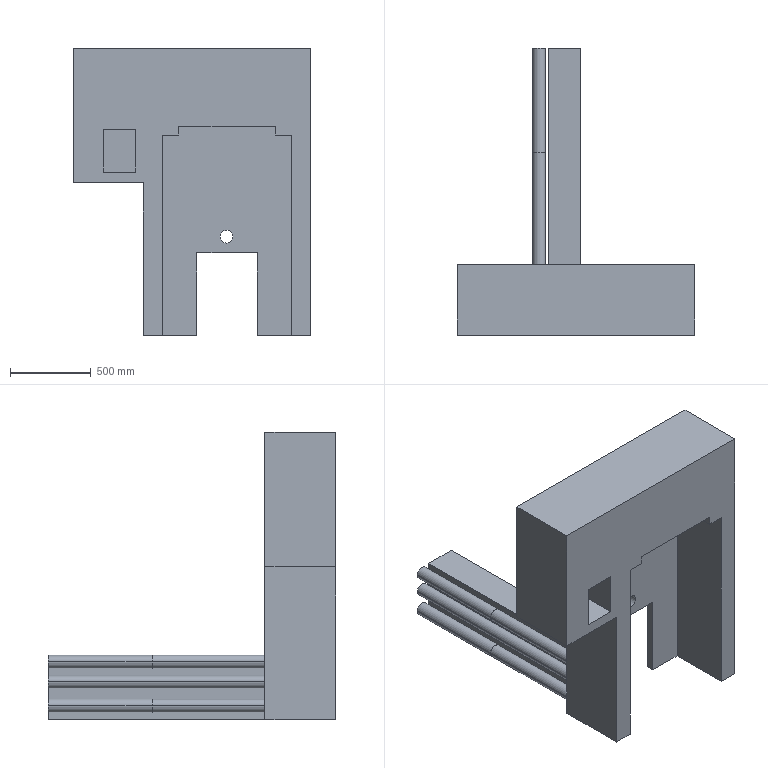Part | STEP file | Boss-Extrude 14 | 1 solid | 45 faces | box 1476 x 1784 x 1786 mm | volume 674067004 mm3 | plane 33 | cylinder 12 | commonest cylinder face diameters 80 x8 79.08 x2 83.019 x2
STEP:
#1=CARTESIAN_POINT('',(-754.337,404.541,3154.64));
#2=VERTEX_POINT('',#1);
#3=CARTESIAN_POINT('',(-754.337,404.541,3234.64));
#4=VERTEX_POINT('',#3);
#5=CARTESIAN_POINT('',(-754.337,404.541,3194.64));
#6=DIRECTION('',(0.,1.,0.));
#7=DIRECTION('',(1.,0.,0.));
#8=AXIS2_PLACEMENT_3D('',#5,#6,#7);
#9=CIRCLE('',#8,40.);
#10=EDGE_CURVE('',#2,#4,#9,.T.);
#11=ORIENTED_EDGE('',*,*,#10,.F.);
#12=CARTESIAN_POINT('',(-754.337,454.541,3154.64));
#13=VERTEX_POINT('',#12);
#14=CARTESIAN_POINT('',(-754.337,63.541,3154.64));
#15=DIRECTION('',(0.,-1.,0.));
#16=VECTOR('',#15,1000.);
#17=LINE('',#14,#16);
#18=EDGE_CURVE('',#13,#2,#17,.T.);
#19=ORIENTED_EDGE('',*,*,#18,.F.);
#20=CARTESIAN_POINT('',(-754.337,454.541,3234.64));
#21=VERTEX_POINT('',#20);
#22=CARTESIAN_POINT('',(-754.337,454.541,3194.64));
#23=DIRECTION('',(0.,1.,0.));
#24=DIRECTION('',(1.,0.,0.));
#25=AXIS2_PLACEMENT_3D('',#22,#23,#24);
#26=CIRCLE('',#25,40.);
#27=EDGE_CURVE('',#13,#21,#26,.T.);
#28=ORIENTED_EDGE('',*,*,#27,.T.);
#29=CARTESIAN_POINT('',(-754.337,63.541,3234.64));
#30=DIRECTION('',(0.,-1.,0.));
#31=VECTOR('',#30,1000.);
#32=LINE('',#29,#31);
#33=EDGE_CURVE('',#21,#4,#32,.T.);
#34=ORIENTED_EDGE('',*,*,#33,.T.);
#35=EDGE_LOOP('',(#11,#19,#28,#34));
#36=FACE_OUTER_BOUND('',#35,.T.);
#37=CARTESIAN_POINT('',(-754.337,63.541,3194.64));
#38=DIRECTION('',(0.,1.,0.));
#39=DIRECTION('',(0.,0.,-1.));
#40=AXIS2_PLACEMENT_3D('',#37,#38,#39);
#41=CYLINDRICAL_SURFACE('',#40,40.);
#42=ADVANCED_FACE('',(#36),#41,.F.);
#43=CARTESIAN_POINT('',(-1157.141,1799.261,2665.873));
#44=VERTEX_POINT('',#43);
#45=CARTESIAN_POINT('',(-1240.161,1799.261,2665.873));
#46=VERTEX_POINT('',#45);
#47=CARTESIAN_POINT('',(-1198.651,1799.261,2665.873));
#48=DIRECTION('',(0.,1.,0.));
#49=DIRECTION('',(1.,0.,0.));
#50=AXIS2_PLACEMENT_3D('',#47,#48,#49);
#51=CIRCLE('',#50,41.51);
#52=EDGE_CURVE('',#44,#46,#51,.T.);
#53=ORIENTED_EDGE('',*,*,#52,.F.);
#54=CARTESIAN_POINT('',(-1157.141,1154.541,2665.873));
#55=VERTEX_POINT('',#54);
#56=CARTESIAN_POINT('',(-1157.141,1799.261,2665.873));
#57=DIRECTION('',(0.,1.,0.));
#58=VECTOR('',#57,1000.);
#59=LINE('',#56,#58);
#60=EDGE_CURVE('',#55,#44,#59,.T.);
#61=ORIENTED_EDGE('',*,*,#60,.F.);
#62=CARTESIAN_POINT('',(-1240.161,1154.541,2665.873));
#63=VERTEX_POINT('',#62);
#64=CARTESIAN_POINT('',(-1198.651,1154.541,2665.873));
#65=DIRECTION('',(0.,1.,0.));
#66=DIRECTION('',(1.,0.,0.));
#67=AXIS2_PLACEMENT_3D('',#64,#65,#66);
#68=CIRCLE('',#67,41.51);
#69=EDGE_CURVE('',#55,#63,#68,.T.);
#70=ORIENTED_EDGE('',*,*,#69,.T.);
#71=CARTESIAN_POINT('',(-1240.161,1799.261,2665.873));
#72=DIRECTION('',(0.,1.,0.));
#73=VECTOR('',#72,1000.);
#74=LINE('',#71,#73);
#75=EDGE_CURVE('',#63,#46,#74,.T.);
#76=ORIENTED_EDGE('',*,*,#75,.T.);
#77=EDGE_LOOP('',(#53,#61,#70,#76));
#78=FACE_OUTER_BOUND('',#77,.T.);
#79=CARTESIAN_POINT('',(-1198.651,1799.261,2665.873));
#80=DIRECTION('',(0.,-1.,0.));
#81=DIRECTION('',(1.,0.,0.));
#82=AXIS2_PLACEMENT_3D('',#79,#80,#81);
#83=CYLINDRICAL_SURFACE('',#82,41.51);
#84=ADVANCED_FACE('',(#78),#83,.T.);
#85=CARTESIAN_POINT('',(-1159.111,1799.261,2938.96));
#86=VERTEX_POINT('',#85);
#87=CARTESIAN_POINT('',(-1238.191,1799.261,2938.96));
#88=VERTEX_POINT('',#87);
#89=CARTESIAN_POINT('',(-1198.651,1799.261,2938.96));
#90=DIRECTION('',(0.,1.,0.));
#91=DIRECTION('',(1.,0.,0.));
#92=AXIS2_PLACEMENT_3D('',#89,#90,#91);
#93=CIRCLE('',#92,39.54);
#94=EDGE_CURVE('',#86,#88,#93,.T.);
#95=ORIENTED_EDGE('',*,*,#94,.F.);
#96=CARTESIAN_POINT('',(-1159.111,1154.541,2938.96));
#97=VERTEX_POINT('',#96);
#98=CARTESIAN_POINT('',(-1159.111,1799.261,2938.96));
#99=DIRECTION('',(0.,1.,0.));
#100=VECTOR('',#99,1000.);
#101=LINE('',#98,#100);
#102=EDGE_CURVE('',#97,#86,#101,.T.);
#103=ORIENTED_EDGE('',*,*,#102,.F.);
#104=CARTESIAN_POINT('',(-1238.191,1154.541,2938.96));
#105=VERTEX_POINT('',#104);
#106=CARTESIAN_POINT('',(-1198.651,1154.541,2938.96));
#107=DIRECTION('',(0.,1.,0.));
#108=DIRECTION('',(1.,0.,0.));
#109=AXIS2_PLACEMENT_3D('',#106,#107,#108);
#110=CIRCLE('',#109,39.54);
#111=EDGE_CURVE('',#97,#105,#110,.T.);
#112=ORIENTED_EDGE('',*,*,#111,.T.);
#113=CARTESIAN_POINT('',(-1238.191,1799.261,2938.96));
#114=DIRECTION('',(0.,1.,0.));
#115=VECTOR('',#114,1000.);
#116=LINE('',#113,#115);
#117=EDGE_CURVE('',#105,#88,#116,.T.);
#118=ORIENTED_EDGE('',*,*,#117,.T.);
#119=EDGE_LOOP('',(#95,#103,#112,#118));
#120=FACE_OUTER_BOUND('',#119,.T.);
#121=CARTESIAN_POINT('',(-1198.651,1799.261,2938.96));
#122=DIRECTION('',(0.,-1.,0.));
#123=DIRECTION('',(1.,0.,0.));
#124=AXIS2_PLACEMENT_3D('',#121,#122,#123);
#125=CYLINDRICAL_SURFACE('',#124,39.54);
#126=ADVANCED_FACE('',(#120),#125,.T.);
#127=CARTESIAN_POINT('',(-1158.651,1799.261,2813.856));
#128=VERTEX_POINT('',#127);
#129=CARTESIAN_POINT('',(-1238.651,1799.261,2813.856));
#130=VERTEX_POINT('',#129);
#131=CARTESIAN_POINT('',(-1198.651,1799.261,2813.856));
#132=DIRECTION('',(0.,1.,0.));
#133=DIRECTION('',(1.,0.,0.));
#134=AXIS2_PLACEMENT_3D('',#131,#132,#133);
#135=CIRCLE('',#134,40.);
#136=EDGE_CURVE('',#128,#130,#135,.T.);
#137=ORIENTED_EDGE('',*,*,#136,.F.);
#138=CARTESIAN_POINT('',(-1158.651,454.541,2813.856));
#139=VERTEX_POINT('',#138);
#140=CARTESIAN_POINT('',(-1158.651,1154.541,2813.856));
#141=DIRECTION('',(0.,1.,0.));
#142=VECTOR('',#141,1000.);
#143=LINE('',#140,#142);
#144=EDGE_CURVE('',#139,#128,#143,.T.);
#145=ORIENTED_EDGE('',*,*,#144,.F.);
#146=CARTESIAN_POINT('',(-1238.651,454.541,2813.856));
#147=VERTEX_POINT('',#146);
#148=CARTESIAN_POINT('',(-1198.651,454.541,2813.856));
#149=DIRECTION('',(0.,1.,0.));
#150=DIRECTION('',(1.,0.,0.));
#151=AXIS2_PLACEMENT_3D('',#148,#149,#150);
#152=CIRCLE('',#151,40.);
#153=EDGE_CURVE('',#139,#147,#152,.T.);
#154=ORIENTED_EDGE('',*,*,#153,.T.);
#155=CARTESIAN_POINT('',(-1238.651,1154.541,2813.856));
#156=DIRECTION('',(0.,1.,0.));
#157=VECTOR('',#156,1000.);
#158=LINE('',#155,#157);
#159=EDGE_CURVE('',#147,#130,#158,.T.);
#160=ORIENTED_EDGE('',*,*,#159,.T.);
#161=EDGE_LOOP('',(#137,#145,#154,#160));
#162=FACE_OUTER_BOUND('',#161,.T.);
#163=CARTESIAN_POINT('',(-1198.651,1154.541,2813.856));
#164=DIRECTION('',(0.,-1.,0.));
#165=DIRECTION('',(1.,0.,0.));
#166=AXIS2_PLACEMENT_3D('',#163,#164,#165);
#167=CYLINDRICAL_SURFACE('',#166,40.);
#168=ADVANCED_FACE('',(#162),#167,.T.);
#169=CARTESIAN_POINT('',(-1158.651,1154.541,2938.96));
#170=VERTEX_POINT('',#169);
#171=CARTESIAN_POINT('',(-1238.651,1154.541,2938.96));
#172=VERTEX_POINT('',#171);
#173=CARTESIAN_POINT('',(-1198.651,1154.541,2938.96));
#174=DIRECTION('',(0.,1.,0.));
#175=DIRECTION('',(1.,0.,0.));
#176=AXIS2_PLACEMENT_3D('',#173,#174,#175);
#177=CIRCLE('',#176,40.);
#178=EDGE_CURVE('',#170,#172,#177,.T.);
#179=ORIENTED_EDGE('',*,*,#178,.F.);
#180=CARTESIAN_POINT('',(-1158.651,454.541,2938.96));
#181=VERTEX_POINT('',#180);
#182=CARTESIAN_POINT('',(-1158.651,1154.541,2938.96));
#183=DIRECTION('',(0.,1.,0.));
#184=VECTOR('',#183,1000.);
#185=LINE('',#182,#184);
#186=EDGE_CURVE('',#181,#170,#185,.T.);
#187=ORIENTED_EDGE('',*,*,#186,.F.);
#188=CARTESIAN_POINT('',(-1238.651,454.541,2938.96));
#189=VERTEX_POINT('',#188);
#190=CARTESIAN_POINT('',(-1198.651,454.541,2938.96));
#191=DIRECTION('',(0.,1.,0.));
#192=DIRECTION('',(1.,0.,0.));
#193=AXIS2_PLACEMENT_3D('',#190,#191,#192);
#194=CIRCLE('',#193,40.);
#195=EDGE_CURVE('',#181,#189,#194,.T.);
#196=ORIENTED_EDGE('',*,*,#195,.T.);
#197=CARTESIAN_POINT('',(-1238.651,1154.541,2938.96));
#198=DIRECTION('',(0.,1.,0.));
#199=VECTOR('',#198,1000.);
#200=LINE('',#197,#199);
#201=EDGE_CURVE('',#189,#172,#200,.T.);
#202=ORIENTED_EDGE('',*,*,#201,.T.);
#203=EDGE_LOOP('',(#179,#187,#196,#202));
#204=FACE_OUTER_BOUND('',#203,.T.);
#205=CARTESIAN_POINT('',(-1198.651,1154.541,2938.96));
#206=DIRECTION('',(0.,-1.,0.));
#207=DIRECTION('',(1.,0.,0.));
#208=AXIS2_PLACEMENT_3D('',#205,#206,#207);
#209=CYLINDRICAL_SURFACE('',#208,40.);
#210=ADVANCED_FACE('',(#204),#209,.T.);
#211=CARTESIAN_POINT('',(-1158.651,1154.541,2665.873));
#212=VERTEX_POINT('',#211);
#213=CARTESIAN_POINT('',(-1238.651,1154.541,2665.873));
#214=VERTEX_POINT('',#213);
#215=CARTESIAN_POINT('',(-1198.651,1154.541,2665.873));
#216=DIRECTION('',(0.,1.,0.));
#217=DIRECTION('',(1.,0.,0.));
#218=AXIS2_PLACEMENT_3D('',#215,#216,#217);
#219=CIRCLE('',#218,40.);
#220=EDGE_CURVE('',#212,#214,#219,.T.);
#221=ORIENTED_EDGE('',*,*,#220,.F.);
#222=CARTESIAN_POINT('',(-1158.651,454.541,2665.873));
#223=VERTEX_POINT('',#222);
#224=CARTESIAN_POINT('',(-1158.651,1154.541,2665.873));
#225=DIRECTION('',(0.,1.,0.));
#226=VECTOR('',#225,1000.);
#227=LINE('',#224,#226);
#228=EDGE_CURVE('',#223,#212,#227,.T.);
#229=ORIENTED_EDGE('',*,*,#228,.F.);
#230=CARTESIAN_POINT('',(-1238.651,454.541,2665.873));
#231=VERTEX_POINT('',#230);
#232=CARTESIAN_POINT('',(-1198.651,454.541,2665.873));
#233=DIRECTION('',(0.,1.,0.));
#234=DIRECTION('',(1.,0.,0.));
#235=AXIS2_PLACEMENT_3D('',#232,#233,#234);
#236=CIRCLE('',#235,40.);
#237=EDGE_CURVE('',#223,#231,#236,.T.);
#238=ORIENTED_EDGE('',*,*,#237,.T.);
#239=CARTESIAN_POINT('',(-1238.651,1154.541,2665.873));
#240=DIRECTION('',(0.,1.,0.));
#241=VECTOR('',#240,1000.);
#242=LINE('',#239,#241);
#243=EDGE_CURVE('',#231,#214,#242,.T.);
#244=ORIENTED_EDGE('',*,*,#243,.T.);
#245=EDGE_LOOP('',(#221,#229,#238,#244));
#246=FACE_OUTER_BOUND('',#245,.T.);
#247=CARTESIAN_POINT('',(-1198.651,1154.541,2665.873));
#248=DIRECTION('',(0.,-1.,0.));
#249=DIRECTION('',(1.,0.,0.));
#250=AXIS2_PLACEMENT_3D('',#247,#248,#249);
#251=CYLINDRICAL_SURFACE('',#250,40.);
#252=ADVANCED_FACE('',(#246),#251,.T.);
#253=CARTESIAN_POINT('',(-1271.238,454.541,2578.5));
#254=VERTEX_POINT('',#253);
#255=CARTESIAN_POINT('',(-1271.238,15.541,2578.5));
#256=VERTEX_POINT('',#255);
#257=CARTESIAN_POINT('',(-1271.238,-467.459,2578.5));
#258=DIRECTION('',(0.,-1.,0.));
#259=VECTOR('',#258,1000.);
#260=LINE('',#257,#259);
#261=EDGE_CURVE('',#254,#256,#260,.T.);
#262=ORIENTED_EDGE('',*,*,#261,.T.);
#263=CARTESIAN_POINT('',(-1271.238,15.541,3528.5));
#264=VERTEX_POINT('',#263);
#265=CARTESIAN_POINT('',(-1271.238,15.541,2578.5));
#266=DIRECTION('',(0.,0.,-1.));
#267=VECTOR('',#266,1000.);
#268=LINE('',#265,#267);
#269=EDGE_CURVE('',#264,#256,#268,.T.);
#270=ORIENTED_EDGE('',*,*,#269,.F.);
#271=CARTESIAN_POINT('',(-1271.238,454.541,3528.5));
#272=VERTEX_POINT('',#271);
#273=CARTESIAN_POINT('',(-1271.238,454.541,3528.5));
#274=DIRECTION('',(0.,-1.,0.));
#275=VECTOR('',#274,1000.);
#276=LINE('',#273,#275);
#277=EDGE_CURVE('',#272,#264,#276,.T.);
#278=ORIENTED_EDGE('',*,*,#277,.F.);
#279=CARTESIAN_POINT('',(-1271.238,454.541,2578.5));
#280=DIRECTION('',(0.,0.,-1.));
#281=VECTOR('',#280,1000.);
#282=LINE('',#279,#281);
#283=EDGE_CURVE('',#272,#254,#282,.T.);
#284=ORIENTED_EDGE('',*,*,#283,.T.);
#285=EDGE_LOOP('',(#262,#270,#278,#284));
#286=FACE_OUTER_BOUND('',#285,.T.);
#287=CARTESIAN_POINT('',(-1271.238,-45.459,2978.5));
#288=DIRECTION('',(1.,0.,0.));
#289=DIRECTION('',(0.,0.,1.));
#290=AXIS2_PLACEMENT_3D('',#287,#288,#289);
#291=PLANE('',#290);
#292=ADVANCED_FACE('',(#286),#291,.F.);
#293=CARTESIAN_POINT('',(-754.337,404.541,3194.64));
#294=DIRECTION('',(0.,1.,0.));
#295=DIRECTION('',(1.,0.,0.));
#296=AXIS2_PLACEMENT_3D('',#293,#294,#295);
#297=CIRCLE('',#296,40.);
#298=EDGE_CURVE('',#4,#2,#297,.T.);
#299=ORIENTED_EDGE('',*,*,#298,.T.);
#300=ORIENTED_EDGE('',*,*,#10,.T.);
#301=EDGE_LOOP('',(#299,#300));
#302=FACE_BOUND('',#301,.T.);
#303=CARTESIAN_POINT('',(-1051.238,404.541,3878.5));
#304=VERTEX_POINT('',#303);
#305=CARTESIAN_POINT('',(-1051.238,404.541,3825.5));
#306=VERTEX_POINT('',#305);
#307=CARTESIAN_POINT('',(-1051.238,404.541,3328.5));
#308=DIRECTION('',(0.,0.,-1.));
#309=VECTOR('',#308,1000.);
#310=LINE('',#307,#309);
#311=EDGE_CURVE('',#304,#306,#310,.T.);
#312=ORIENTED_EDGE('',*,*,#311,.T.);
#313=CARTESIAN_POINT('',(-1151.238,404.541,3825.5));
#314=VERTEX_POINT('',#313);
#315=CARTESIAN_POINT('',(-1051.238,404.541,3825.5));
#316=DIRECTION('',(1.,0.,0.));
#317=VECTOR('',#316,1000.);
#318=LINE('',#315,#317);
#319=EDGE_CURVE('',#314,#306,#318,.T.);
#320=ORIENTED_EDGE('',*,*,#319,.F.);
#321=CARTESIAN_POINT('',(-1151.238,404.541,2578.5));
#322=VERTEX_POINT('',#321);
#323=CARTESIAN_POINT('',(-1151.238,404.541,3875.5));
#324=DIRECTION('',(0.,0.,-1.));
#325=VECTOR('',#324,1000.);
#326=LINE('',#323,#325);
#327=EDGE_CURVE('',#314,#322,#326,.T.);
#328=ORIENTED_EDGE('',*,*,#327,.T.);
#329=CARTESIAN_POINT('',(-938.738,404.541,2578.5));
#330=VERTEX_POINT('',#329);
#331=CARTESIAN_POINT('',(-451.238,404.541,2578.5));
#332=DIRECTION('',(1.,0.,0.));
#333=VECTOR('',#332,1000.);
#334=LINE('',#331,#333);
#335=EDGE_CURVE('',#322,#330,#334,.T.);
#336=ORIENTED_EDGE('',*,*,#335,.T.);
#337=CARTESIAN_POINT('',(-938.738,404.541,3094.));
#338=VERTEX_POINT('',#337);
#339=CARTESIAN_POINT('',(-938.738,404.541,3328.5));
#340=DIRECTION('',(0.,0.,1.));
#341=VECTOR('',#340,1000.);
#342=LINE('',#339,#341);
#343=EDGE_CURVE('',#330,#338,#342,.T.);
#344=ORIENTED_EDGE('',*,*,#343,.T.);
#345=CARTESIAN_POINT('',(-563.738,404.541,3094.));
#346=VERTEX_POINT('',#345);
#347=CARTESIAN_POINT('',(-451.238,404.541,3094.));
#348=DIRECTION('',(1.,0.,0.));
#349=VECTOR('',#348,1000.);
#350=LINE('',#347,#349);
#351=EDGE_CURVE('',#338,#346,#350,.T.);
#352=ORIENTED_EDGE('',*,*,#351,.T.);
#353=CARTESIAN_POINT('',(-563.738,404.541,2578.5));
#354=VERTEX_POINT('',#353);
#355=CARTESIAN_POINT('',(-563.738,404.541,3328.5));
#356=DIRECTION('',(0.,0.,-1.));
#357=VECTOR('',#356,1000.);
#358=LINE('',#355,#357);
#359=EDGE_CURVE('',#346,#354,#358,.T.);
#360=ORIENTED_EDGE('',*,*,#359,.T.);
#361=CARTESIAN_POINT('',(-351.238,404.541,2578.5));
#362=VERTEX_POINT('',#361);
#363=CARTESIAN_POINT('',(-451.238,404.541,2578.5));
#364=DIRECTION('',(1.,0.,0.));
#365=VECTOR('',#364,1000.);
#366=LINE('',#363,#365);
#367=EDGE_CURVE('',#354,#362,#366,.T.);
#368=ORIENTED_EDGE('',*,*,#367,.T.);
#369=CARTESIAN_POINT('',(-351.238,404.541,3825.5));
#370=VERTEX_POINT('',#369);
#371=CARTESIAN_POINT('',(-351.238,404.541,3875.5));
#372=DIRECTION('',(0.,0.,-1.));
#373=VECTOR('',#372,1000.);
#374=LINE('',#371,#373);
#375=EDGE_CURVE('',#370,#362,#374,.T.);
#376=ORIENTED_EDGE('',*,*,#375,.F.);
#377=CARTESIAN_POINT('',(-451.238,404.541,3825.5));
#378=VERTEX_POINT('',#377);
#379=CARTESIAN_POINT('',(-351.238,404.541,3825.5));
#380=DIRECTION('',(1.,0.,0.));
#381=VECTOR('',#380,1000.);
#382=LINE('',#379,#381);
#383=EDGE_CURVE('',#378,#370,#382,.T.);
#384=ORIENTED_EDGE('',*,*,#383,.F.);
#385=CARTESIAN_POINT('',(-451.238,404.541,3878.5));
#386=VERTEX_POINT('',#385);
#387=CARTESIAN_POINT('',(-451.238,404.541,3328.5));
#388=DIRECTION('',(0.,0.,-1.));
#389=VECTOR('',#388,1000.);
#390=LINE('',#387,#389);
#391=EDGE_CURVE('',#386,#378,#390,.T.);
#392=ORIENTED_EDGE('',*,*,#391,.F.);
#393=CARTESIAN_POINT('',(-1051.238,404.541,3878.5));
#394=DIRECTION('',(1.,0.,0.));
#395=VECTOR('',#394,1000.);
#396=LINE('',#393,#395);
#397=EDGE_CURVE('',#304,#386,#396,.T.);
#398=ORIENTED_EDGE('',*,*,#397,.F.);
#399=EDGE_LOOP('',(#312,#320,#328,#336,#344,#352,#360,#368,#376,#384,#392,#398));
#400=FACE_OUTER_BOUND('',#399,.T.);
#401=CARTESIAN_POINT('',(-451.238,404.541,3328.5));
#402=DIRECTION('',(0.,1.,0.));
#403=DIRECTION('',(-1.,0.,0.));
#404=AXIS2_PLACEMENT_3D('',#401,#402,#403);
#405=PLANE('',#404);
#406=ADVANCED_FACE('',(#302,#400),#405,.F.);
#407=CARTESIAN_POINT('',(-1151.238,15.541,3825.5));
#408=VERTEX_POINT('',#407);
#409=CARTESIAN_POINT('',(-1151.238,404.541,3825.5));
#410=DIRECTION('',(0.,1.,0.));
#411=VECTOR('',#410,1000.);
#412=LINE('',#409,#411);
#413=EDGE_CURVE('',#408,#314,#412,.T.);
#414=ORIENTED_EDGE('',*,*,#413,.F.);
#415=CARTESIAN_POINT('',(-1151.238,15.541,2578.5));
#416=VERTEX_POINT('',#415);
#417=CARTESIAN_POINT('',(-1151.238,15.541,3825.5));
#418=DIRECTION('',(0.,0.,1.));
#419=VECTOR('',#418,1000.);
#420=LINE('',#417,#419);
#421=EDGE_CURVE('',#416,#408,#420,.T.);
#422=ORIENTED_EDGE('',*,*,#421,.F.);
#423=CARTESIAN_POINT('',(-1151.238,404.541,2578.5));
#424=DIRECTION('',(0.,1.,0.));
#425=VECTOR('',#424,1000.);
#426=LINE('',#423,#425);
#427=EDGE_CURVE('',#416,#322,#426,.T.);
#428=ORIENTED_EDGE('',*,*,#427,.T.);
#429=ORIENTED_EDGE('',*,*,#327,.F.);
#430=EDGE_LOOP('',(#414,#422,#428,#429));
#431=FACE_OUTER_BOUND('',#430,.T.);
#432=CARTESIAN_POINT('',(-1151.238,404.541,3875.5));
#433=DIRECTION('',(-1.,0.,0.));
#434=DIRECTION('',(0.,0.,-1.));
#435=AXIS2_PLACEMENT_3D('',#432,#433,#434);
#436=PLANE('',#435);
#437=ADVANCED_FACE('',(#431),#436,.F.);
#438=CARTESIAN_POINT('',(-351.238,15.541,2578.5));
#439=VERTEX_POINT('',#438);
#440=CARTESIAN_POINT('',(-351.238,404.541,2578.5));
#441=DIRECTION('',(0.,-1.,0.));
#442=VECTOR('',#441,1000.);
#443=LINE('',#440,#442);
#444=EDGE_CURVE('',#362,#439,#443,.T.);
#445=ORIENTED_EDGE('',*,*,#444,.T.);
#446=CARTESIAN_POINT('',(-351.238,15.541,3825.5));
#447=VERTEX_POINT('',#446);
#448=CARTESIAN_POINT('',(-351.238,15.541,2578.5));
#449=DIRECTION('',(0.,0.,-1.));
#450=VECTOR('',#449,1000.);
#451=LINE('',#448,#450);
#452=EDGE_CURVE('',#447,#439,#451,.T.);
#453=ORIENTED_EDGE('',*,*,#452,.F.);
#454=CARTESIAN_POINT('',(-351.238,-467.459,3825.5));
#455=DIRECTION('',(0.,-1.,0.));
#456=VECTOR('',#455,1000.);
#457=LINE('',#454,#456);
#458=EDGE_CURVE('',#370,#447,#457,.T.);
#459=ORIENTED_EDGE('',*,*,#458,.F.);
#460=ORIENTED_EDGE('',*,*,#375,.T.);
#461=EDGE_LOOP('',(#445,#453,#459,#460));
#462=FACE_OUTER_BOUND('',#461,.T.);
#463=CARTESIAN_POINT('',(-351.238,404.541,3875.5));
#464=DIRECTION('',(1.,0.,0.));
#465=DIRECTION('',(0.,0.,1.));
#466=AXIS2_PLACEMENT_3D('',#463,#464,#465);
#467=PLANE('',#466);
#468=ADVANCED_FACE('',(#462),#467,.F.);
#469=CARTESIAN_POINT('',(-451.238,15.541,3825.5));
#470=VERTEX_POINT('',#469);
#471=CARTESIAN_POINT('',(-451.238,404.541,3825.5));
#472=DIRECTION('',(0.,1.,0.));
#473=VECTOR('',#472,1000.);
#474=LINE('',#471,#473);
#475=EDGE_CURVE('',#470,#378,#474,.T.);
#476=ORIENTED_EDGE('',*,*,#475,.F.);
#477=CARTESIAN_POINT('',(-451.238,15.541,3878.5));
#478=VERTEX_POINT('',#477);
#479=CARTESIAN_POINT('',(-451.238,15.541,3825.5));
#480=DIRECTION('',(0.,0.,-1.));
#481=VECTOR('',#480,1000.);
#482=LINE('',#479,#481);
#483=EDGE_CURVE('',#478,#470,#482,.T.);
#484=ORIENTED_EDGE('',*,*,#483,.F.);
#485=CARTESIAN_POINT('',(-451.238,404.541,3878.5));
#486=DIRECTION('',(0.,-1.,0.));
#487=VECTOR('',#486,1000.);
#488=LINE('',#485,#487);
#489=EDGE_CURVE('',#386,#478,#488,.T.);
#490=ORIENTED_EDGE('',*,*,#489,.F.);
#491=ORIENTED_EDGE('',*,*,#391,.T.);
#492=EDGE_LOOP('',(#476,#484,#490,#491));
#493=FACE_OUTER_BOUND('',#492,.T.);
#494=CARTESIAN_POINT('',(-451.238,404.541,3328.5));
#495=DIRECTION('',(1.,0.,0.));
#496=DIRECTION('',(0.,0.,1.));
#497=AXIS2_PLACEMENT_3D('',#494,#495,#496);
#498=PLANE('',#497);
#499=ADVANCED_FACE('',(#493),#498,.F.);
#500=ORIENTED_EDGE('',*,*,#427,.F.);
#501=CARTESIAN_POINT('',(-1151.238,15.541,2578.5));
#502=DIRECTION('',(1.,0.,0.));
#503=VECTOR('',#502,1000.);
#504=LINE('',#501,#503);
#505=EDGE_CURVE('',#256,#416,#504,.T.);
#506=ORIENTED_EDGE('',*,*,#505,.F.);
#507=ORIENTED_EDGE('',*,*,#261,.F.);
#508=CARTESIAN_POINT('',(-1138.738,454.541,2578.5));
#509=VERTEX_POINT('',#508);
#510=CARTESIAN_POINT('',(-1101.238,454.541,2578.5));
#511=DIRECTION('',(-1.,0.,0.));
#512=VECTOR('',#511,1000.);
#513=LINE('',#510,#512);
#514=EDGE_CURVE('',#509,#254,#513,.T.);
#515=ORIENTED_EDGE('',*,*,#514,.F.);
#516=CARTESIAN_POINT('',(-1138.738,1799.261,2578.5));
#517=VERTEX_POINT('',#516);
#518=CARTESIAN_POINT('',(-1138.738,1154.541,2578.5));
#519=DIRECTION('',(0.,-1.,0.));
#520=VECTOR('',#519,1000.);
#521=LINE('',#518,#520);
#522=EDGE_CURVE('',#517,#509,#521,.T.);
#523=ORIENTED_EDGE('',*,*,#522,.F.);
#524=CARTESIAN_POINT('',(-938.738,1799.261,2578.5));
#525=VERTEX_POINT('',#524);
#526=CARTESIAN_POINT('',(-1138.738,1799.261,2578.5));
#527=DIRECTION('',(-1.,0.,0.));
#528=VECTOR('',#527,1000.);
#529=LINE('',#526,#528);
#530=EDGE_CURVE('',#525,#517,#529,.T.);
#531=ORIENTED_EDGE('',*,*,#530,.F.);
#532=CARTESIAN_POINT('',(-938.738,19.541,2578.5));
#533=DIRECTION('',(0.,1.,0.));
#534=VECTOR('',#533,1000.);
#535=LINE('',#532,#534);
#536=EDGE_CURVE('',#330,#525,#535,.T.);
#537=ORIENTED_EDGE('',*,*,#536,.F.);
#538=ORIENTED_EDGE('',*,*,#335,.F.);
#539=EDGE_LOOP('',(#500,#506,#507,#515,#523,#531,#537,#538));
#540=FACE_OUTER_BOUND('',#539,.T.);
#541=CARTESIAN_POINT('',(-1101.238,454.541,2578.5));
#542=DIRECTION('',(0.,0.,1.));
#543=DIRECTION('',(-1.,0.,0.));
#544=AXIS2_PLACEMENT_3D('',#541,#542,#543);
#545=PLANE('',#544);
#546=ADVANCED_FACE('',(#540),#545,.F.);
#547=CARTESIAN_POINT('',(-231.238,15.541,2578.5));
#548=VERTEX_POINT('',#547);
#549=CARTESIAN_POINT('',(-231.238,454.541,2578.5));
#550=VERTEX_POINT('',#549);
#551=CARTESIAN_POINT('',(-231.238,454.541,2578.5));
#552=DIRECTION('',(0.,1.,0.));
#553=VECTOR('',#552,1000.);
#554=LINE('',#551,#553);
#555=EDGE_CURVE('',#548,#550,#554,.T.);
#556=ORIENTED_EDGE('',*,*,#555,.F.);
#557=CARTESIAN_POINT('',(-231.238,15.541,2578.5));
#558=DIRECTION('',(1.,0.,0.));
#559=VECTOR('',#558,1000.);
#560=LINE('',#557,#559);
#561=EDGE_CURVE('',#439,#548,#560,.T.);
#562=ORIENTED_EDGE('',*,*,#561,.F.);
#563=ORIENTED_EDGE('',*,*,#444,.F.);
#564=ORIENTED_EDGE('',*,*,#367,.F.);
#565=CARTESIAN_POINT('',(-563.738,454.541,2578.5));
#566=VERTEX_POINT('',#565);
#567=CARTESIAN_POINT('',(-563.738,19.541,2578.5));
#568=DIRECTION('',(0.,1.,0.));
#569=VECTOR('',#568,1000.);
#570=LINE('',#567,#569);
#571=EDGE_CURVE('',#354,#566,#570,.T.);
#572=ORIENTED_EDGE('',*,*,#571,.T.);
#573=CARTESIAN_POINT('',(-1101.238,454.541,2578.5));
#574=DIRECTION('',(-1.,0.,0.));
#575=VECTOR('',#574,1000.);
#576=LINE('',#573,#575);
#577=EDGE_CURVE('',#550,#566,#576,.T.);
#578=ORIENTED_EDGE('',*,*,#577,.F.);
#579=EDGE_LOOP('',(#556,#562,#563,#564,#572,#578));
#580=FACE_OUTER_BOUND('',#579,.T.);
#581=CARTESIAN_POINT('',(-1101.238,454.541,2578.5));
#582=DIRECTION('',(0.,0.,1.));
#583=DIRECTION('',(-1.,0.,0.));
#584=AXIS2_PLACEMENT_3D('',#581,#582,#583);
#585=PLANE('',#584);
#586=ADVANCED_FACE('',(#580),#585,.F.);
#587=CARTESIAN_POINT('',(-754.337,454.541,3194.64));
#588=DIRECTION('',(0.,1.,0.));
#589=DIRECTION('',(1.,0.,0.));
#590=AXIS2_PLACEMENT_3D('',#587,#588,#589);
#591=CIRCLE('',#590,40.);
#592=EDGE_CURVE('',#21,#13,#591,.T.);
#593=ORIENTED_EDGE('',*,*,#592,.F.);
#594=ORIENTED_EDGE('',*,*,#27,.F.);
#595=EDGE_LOOP('',(#593,#594));
#596=FACE_BOUND('',#595,.T.);
#597=CARTESIAN_POINT('',(-1198.651,454.541,2813.856));
#598=DIRECTION('',(0.,1.,0.));
#599=DIRECTION('',(1.,0.,0.));
#600=AXIS2_PLACEMENT_3D('',#597,#598,#599);
#601=CIRCLE('',#600,40.);
#602=EDGE_CURVE('',#147,#139,#601,.T.);
#603=ORIENTED_EDGE('',*,*,#602,.F.);
#604=ORIENTED_EDGE('',*,*,#153,.F.);
#605=EDGE_LOOP('',(#603,#604));
#606=FACE_BOUND('',#605,.T.);
#607=CARTESIAN_POINT('',(-1198.651,454.541,2938.96));
#608=DIRECTION('',(0.,1.,0.));
#609=DIRECTION('',(1.,0.,0.));
#610=AXIS2_PLACEMENT_3D('',#607,#608,#609);
#611=CIRCLE('',#610,40.);
#612=EDGE_CURVE('',#189,#181,#611,.T.);
#613=ORIENTED_EDGE('',*,*,#612,.F.);
#614=ORIENTED_EDGE('',*,*,#195,.F.);
#615=EDGE_LOOP('',(#613,#614));
#616=FACE_BOUND('',#615,.T.);
#617=CARTESIAN_POINT('',(-1198.651,454.541,2665.873));
#618=DIRECTION('',(0.,1.,0.));
#619=DIRECTION('',(1.,0.,0.));
#620=AXIS2_PLACEMENT_3D('',#617,#618,#619);
#621=CIRCLE('',#620,40.);
#622=EDGE_CURVE('',#231,#223,#621,.T.);
#623=ORIENTED_EDGE('',*,*,#622,.F.);
#624=ORIENTED_EDGE('',*,*,#237,.F.);
#625=EDGE_LOOP('',(#623,#624));
#626=FACE_BOUND('',#625,.T.);
#627=CARTESIAN_POINT('',(-938.738,454.541,2978.5));
#628=VERTEX_POINT('',#627);
#629=CARTESIAN_POINT('',(-938.738,454.541,3094.));
#630=VERTEX_POINT('',#629);
#631=CARTESIAN_POINT('',(-938.738,454.541,2978.5));
#632=DIRECTION('',(0.,0.,1.));
#633=VECTOR('',#632,1000.);
#634=LINE('',#631,#633);
#635=EDGE_CURVE('',#628,#630,#634,.T.);
#636=ORIENTED_EDGE('',*,*,#635,.F.);
#637=CARTESIAN_POINT('',(-1138.738,454.541,2978.5));
#638=VERTEX_POINT('',#637);
#639=CARTESIAN_POINT('',(-938.738,454.541,2978.5));
#640=DIRECTION('',(-1.,0.,0.));
#641=VECTOR('',#640,1000.);
#642=LINE('',#639,#641);
#643=EDGE_CURVE('',#628,#638,#642,.T.);
#644=ORIENTED_EDGE('',*,*,#643,.T.);
#645=CARTESIAN_POINT('',(-1138.738,454.541,2578.5));
#646=DIRECTION('',(0.,0.,1.));
#647=VECTOR('',#646,1000.);
#648=LINE('',#645,#647);
#649=EDGE_CURVE('',#509,#638,#648,.T.);
#650=ORIENTED_EDGE('',*,*,#649,.F.);
#651=ORIENTED_EDGE('',*,*,#514,.T.);
#652=ORIENTED_EDGE('',*,*,#283,.F.);
#653=CARTESIAN_POINT('',(-1707.238,454.541,3528.5));
#654=VERTEX_POINT('',#653);
#655=CARTESIAN_POINT('',(-1571.238,454.541,3528.5));
#656=DIRECTION('',(1.,0.,0.));
#657=VECTOR('',#656,1000.);
#658=LINE('',#655,#657);
#659=EDGE_CURVE('',#654,#272,#658,.T.);
#660=ORIENTED_EDGE('',*,*,#659,.F.);
#661=CARTESIAN_POINT('',(-1707.238,454.541,4364.5));
#662=VERTEX_POINT('',#661);
#663=CARTESIAN_POINT('',(-1707.238,454.541,2978.5));
#664=DIRECTION('',(0.,0.,-1.));
#665=VECTOR('',#664,1000.);
#666=LINE('',#663,#665);
#667=EDGE_CURVE('',#662,#654,#666,.T.);
#668=ORIENTED_EDGE('',*,*,#667,.F.);
#669=CARTESIAN_POINT('',(-231.238,454.541,4364.5));
#670=VERTEX_POINT('',#669);
#671=CARTESIAN_POINT('',(-1571.238,454.541,4364.5));
#672=DIRECTION('',(-1.,0.,0.));
#673=VECTOR('',#672,1000.);
#674=LINE('',#671,#673);
#675=EDGE_CURVE('',#670,#662,#674,.T.);
#676=ORIENTED_EDGE('',*,*,#675,.F.);
#677=CARTESIAN_POINT('',(-231.238,454.541,3928.5));
#678=DIRECTION('',(0.,0.,1.));
#679=VECTOR('',#678,1000.);
#680=LINE('',#677,#679);
#681=EDGE_CURVE('',#550,#670,#680,.T.);
#682=ORIENTED_EDGE('',*,*,#681,.F.);
#683=ORIENTED_EDGE('',*,*,#577,.T.);
#684=CARTESIAN_POINT('',(-563.738,454.541,3094.));
#685=VERTEX_POINT('',#684);
#686=CARTESIAN_POINT('',(-563.738,454.541,2978.5));
#687=DIRECTION('',(0.,0.,-1.));
#688=VECTOR('',#687,1000.);
#689=LINE('',#686,#688);
#690=EDGE_CURVE('',#685,#566,#689,.T.);
#691=ORIENTED_EDGE('',*,*,#690,.F.);
#692=CARTESIAN_POINT('',(-751.238,454.541,3094.));
#693=DIRECTION('',(1.,0.,0.));
#694=VECTOR('',#693,1000.);
#695=LINE('',#692,#694);
#696=EDGE_CURVE('',#630,#685,#695,.T.);
#697=ORIENTED_EDGE('',*,*,#696,.F.);
#698=EDGE_LOOP('',(#636,#644,#650,#651,#652,#660,#668,#676,#682,#683,#691,#697));
#699=FACE_OUTER_BOUND('',#698,.T.);
#700=CARTESIAN_POINT('',(-751.238,454.541,2978.5));
#701=DIRECTION('',(0.,1.,0.));
#702=DIRECTION('',(-1.,0.,0.));
#703=AXIS2_PLACEMENT_3D('',#700,#701,#702);
#704=PLANE('',#703);
#705=ADVANCED_FACE('',(#596,#606,#616,#626,#699),#704,.T.);
#706=CARTESIAN_POINT('',(-1051.238,15.541,3878.5));
#707=VERTEX_POINT('',#706);
#708=CARTESIAN_POINT('',(-1051.238,-45.459,3878.5));
#709=DIRECTION('',(0.,1.,0.));
#710=VECTOR('',#709,1000.);
#711=LINE('',#708,#710);
#712=EDGE_CURVE('',#707,#304,#711,.T.);
#713=ORIENTED_EDGE('',*,*,#712,.F.);
#714=CARTESIAN_POINT('',(-1051.238,15.541,3825.5));
#715=VERTEX_POINT('',#714);
#716=CARTESIAN_POINT('',(-1051.238,15.541,3878.5));
#717=DIRECTION('',(0.,0.,1.));
#718=VECTOR('',#717,1000.);
#719=LINE('',#716,#718);
#720=EDGE_CURVE('',#715,#707,#719,.T.);
#721=ORIENTED_EDGE('',*,*,#720,.F.);
#722=CARTESIAN_POINT('',(-1051.238,-467.459,3825.5));
#723=DIRECTION('',(0.,-1.,0.));
#724=VECTOR('',#723,1000.);
#725=LINE('',#722,#724);
#726=EDGE_CURVE('',#306,#715,#725,.T.);
#727=ORIENTED_EDGE('',*,*,#726,.F.);
#728=ORIENTED_EDGE('',*,*,#311,.F.);
#729=EDGE_LOOP('',(#713,#721,#727,#728));
#730=FACE_OUTER_BOUND('',#729,.T.);
#731=CARTESIAN_POINT('',(-1051.238,404.541,3328.5));
#732=DIRECTION('',(-1.,0.,0.));
#733=DIRECTION('',(0.,0.,-1.));
#734=AXIS2_PLACEMENT_3D('',#731,#732,#733);
#735=PLANE('',#734);
#736=ADVANCED_FACE('',(#730),#735,.F.);
#737=CARTESIAN_POINT('',(-938.738,19.541,3094.));
#738=DIRECTION('',(0.,1.,0.));
#739=VECTOR('',#738,1000.);
#740=LINE('',#737,#739);
#741=EDGE_CURVE('',#338,#630,#740,.T.);
#742=ORIENTED_EDGE('',*,*,#741,.T.);
#743=ORIENTED_EDGE('',*,*,#696,.T.);
#744=CARTESIAN_POINT('',(-563.738,19.541,3094.));
#745=DIRECTION('',(0.,1.,0.));
#746=VECTOR('',#745,1000.);
#747=LINE('',#744,#746);
#748=EDGE_CURVE('',#346,#685,#747,.T.);
#749=ORIENTED_EDGE('',*,*,#748,.F.);
#750=ORIENTED_EDGE('',*,*,#351,.F.);
#751=EDGE_LOOP('',(#742,#743,#749,#750));
#752=FACE_OUTER_BOUND('',#751,.T.);
#753=CARTESIAN_POINT('',(-751.238,19.541,3094.));
#754=DIRECTION('',(0.,0.,1.));
#755=DIRECTION('',(-1.,0.,0.));
#756=AXIS2_PLACEMENT_3D('',#753,#754,#755);
#757=PLANE('',#756);
#758=ADVANCED_FACE('',(#752),#757,.F.);
#759=ORIENTED_EDGE('',*,*,#536,.T.);
#760=CARTESIAN_POINT('',(-938.738,1799.261,2978.5));
#761=VERTEX_POINT('',#760);
#762=CARTESIAN_POINT('',(-938.738,1799.261,2578.5));
#763=DIRECTION('',(0.,0.,-1.));
#764=VECTOR('',#763,1000.);
#765=LINE('',#762,#764);
#766=EDGE_CURVE('',#761,#525,#765,.T.);
#767=ORIENTED_EDGE('',*,*,#766,.F.);
#768=CARTESIAN_POINT('',(-938.738,454.541,2978.5));
#769=DIRECTION('',(0.,1.,0.));
#770=VECTOR('',#769,1000.);
#771=LINE('',#768,#770);
#772=EDGE_CURVE('',#628,#761,#771,.T.);
#773=ORIENTED_EDGE('',*,*,#772,.F.);
#774=ORIENTED_EDGE('',*,*,#635,.T.);
#775=ORIENTED_EDGE('',*,*,#741,.F.);
#776=ORIENTED_EDGE('',*,*,#343,.F.);
#777=EDGE_LOOP('',(#759,#767,#773,#774,#775,#776));
#778=FACE_OUTER_BOUND('',#777,.T.);
#779=CARTESIAN_POINT('',(-938.738,19.541,2978.5));
#780=DIRECTION('',(-1.,0.,0.));
#781=DIRECTION('',(0.,0.,-1.));
#782=AXIS2_PLACEMENT_3D('',#779,#780,#781);
#783=PLANE('',#782);
#784=ADVANCED_FACE('',(#778),#783,.F.);
#785=ORIENTED_EDGE('',*,*,#748,.T.);
#786=ORIENTED_EDGE('',*,*,#690,.T.);
#787=ORIENTED_EDGE('',*,*,#571,.F.);
#788=ORIENTED_EDGE('',*,*,#359,.F.);
#789=EDGE_LOOP('',(#785,#786,#787,#788));
#790=FACE_OUTER_BOUND('',#789,.T.);
#791=CARTESIAN_POINT('',(-563.738,19.541,2978.5));
#792=DIRECTION('',(1.,0.,0.));
#793=DIRECTION('',(0.,0.,1.));
#794=AXIS2_PLACEMENT_3D('',#791,#792,#793);
#795=PLANE('',#794);
#796=ADVANCED_FACE('',(#790),#795,.F.);
#797=CARTESIAN_POINT('',(-451.238,15.541,3878.5));
#798=DIRECTION('',(1.,0.,0.));
#799=VECTOR('',#798,1000.);
#800=LINE('',#797,#799);
#801=EDGE_CURVE('',#707,#478,#800,.T.);
#802=ORIENTED_EDGE('',*,*,#801,.F.);
#803=ORIENTED_EDGE('',*,*,#712,.T.);
#804=ORIENTED_EDGE('',*,*,#397,.T.);
#805=ORIENTED_EDGE('',*,*,#489,.T.);
#806=EDGE_LOOP('',(#802,#803,#804,#805));
#807=FACE_OUTER_BOUND('',#806,.T.);
#808=CARTESIAN_POINT('',(-751.238,-45.459,3878.5));
#809=DIRECTION('',(0.,0.,-1.));
#810=DIRECTION('',(1.,0.,0.));
#811=AXIS2_PLACEMENT_3D('',#808,#809,#810);
#812=PLANE('',#811);
#813=ADVANCED_FACE('',(#807),#812,.T.);
#814=ORIENTED_EDGE('',*,*,#458,.T.);
#815=CARTESIAN_POINT('',(-351.238,15.541,3825.5));
#816=DIRECTION('',(1.,0.,0.));
#817=VECTOR('',#816,1000.);
#818=LINE('',#815,#817);
#819=EDGE_CURVE('',#470,#447,#818,.T.);
#820=ORIENTED_EDGE('',*,*,#819,.F.);
#821=ORIENTED_EDGE('',*,*,#475,.T.);
#822=ORIENTED_EDGE('',*,*,#383,.T.);
#823=EDGE_LOOP('',(#814,#820,#821,#822));
#824=FACE_OUTER_BOUND('',#823,.T.);
#825=CARTESIAN_POINT('',(-751.238,-45.459,3825.5));
#826=DIRECTION('',(0.,0.,1.));
#827=DIRECTION('',(-1.,0.,0.));
#828=AXIS2_PLACEMENT_3D('',#825,#826,#827);
#829=PLANE('',#828);
#830=ADVANCED_FACE('',(#824),#829,.F.);
#831=ORIENTED_EDGE('',*,*,#726,.T.);
#832=CARTESIAN_POINT('',(-1051.238,15.541,3825.5));
#833=DIRECTION('',(1.,0.,0.));
#834=VECTOR('',#833,1000.);
#835=LINE('',#832,#834);
#836=EDGE_CURVE('',#408,#715,#835,.T.);
#837=ORIENTED_EDGE('',*,*,#836,.F.);
#838=ORIENTED_EDGE('',*,*,#413,.T.);
#839=ORIENTED_EDGE('',*,*,#319,.T.);
#840=EDGE_LOOP('',(#831,#837,#838,#839));
#841=FACE_OUTER_BOUND('',#840,.T.);
#842=CARTESIAN_POINT('',(-751.238,-45.459,3825.5));
#843=DIRECTION('',(0.,0.,1.));
#844=DIRECTION('',(-1.,0.,0.));
#845=AXIS2_PLACEMENT_3D('',#842,#843,#844);
#846=PLANE('',#845);
#847=ADVANCED_FACE('',(#841),#846,.F.);
#848=ORIENTED_EDGE('',*,*,#681,.T.);
#849=CARTESIAN_POINT('',(-231.238,15.541,4364.5));
#850=VERTEX_POINT('',#849);
#851=CARTESIAN_POINT('',(-231.238,454.541,4364.5));
#852=DIRECTION('',(0.,1.,0.));
#853=VECTOR('',#852,1000.);
#854=LINE('',#851,#853);
#855=EDGE_CURVE('',#850,#670,#854,.T.);
#856=ORIENTED_EDGE('',*,*,#855,.F.);
#857=CARTESIAN_POINT('',(-231.238,15.541,3928.5));
#858=DIRECTION('',(0.,0.,1.));
#859=VECTOR('',#858,1000.);
#860=LINE('',#857,#859);
#861=EDGE_CURVE('',#548,#850,#860,.T.);
#862=ORIENTED_EDGE('',*,*,#861,.F.);
#863=ORIENTED_EDGE('',*,*,#555,.T.);
#864=EDGE_LOOP('',(#848,#856,#862,#863));
#865=FACE_OUTER_BOUND('',#864,.T.);
#866=CARTESIAN_POINT('',(-231.238,-45.459,2978.5));
#867=DIRECTION('',(-1.,0.,0.));
#868=DIRECTION('',(0.,0.,-1.));
#869=AXIS2_PLACEMENT_3D('',#866,#867,#868);
#870=PLANE('',#869);
#871=ADVANCED_FACE('',(#865),#870,.F.);
#872=ORIENTED_EDGE('',*,*,#277,.T.);
#873=CARTESIAN_POINT('',(-1707.238,15.541,3528.5));
#874=VERTEX_POINT('',#873);
#875=CARTESIAN_POINT('',(-1271.238,15.541,3528.5));
#876=DIRECTION('',(1.,0.,0.));
#877=VECTOR('',#876,1000.);
#878=LINE('',#875,#877);
#879=EDGE_CURVE('',#874,#264,#878,.T.);
#880=ORIENTED_EDGE('',*,*,#879,.F.);
#881=CARTESIAN_POINT('',(-1707.238,454.541,3528.5));
#882=DIRECTION('',(0.,-1.,0.));
#883=VECTOR('',#882,1000.);
#884=LINE('',#881,#883);
#885=EDGE_CURVE('',#654,#874,#884,.T.);
#886=ORIENTED_EDGE('',*,*,#885,.F.);
#887=ORIENTED_EDGE('',*,*,#659,.T.);
#888=EDGE_LOOP('',(#872,#880,#886,#887));
#889=FACE_OUTER_BOUND('',#888,.T.);
#890=CARTESIAN_POINT('',(-1571.238,454.541,3528.5));
#891=DIRECTION('',(0.,0.,1.));
#892=DIRECTION('',(-1.,0.,0.));
#893=AXIS2_PLACEMENT_3D('',#890,#891,#892);
#894=PLANE('',#893);
#895=ADVANCED_FACE('',(#889),#894,.F.);
#896=CARTESIAN_POINT('',(-1707.238,15.541,4364.5));
#897=VERTEX_POINT('',#896);
#898=CARTESIAN_POINT('',(-1707.238,15.541,2978.5));
#899=DIRECTION('',(0.,0.,-1.));
#900=VECTOR('',#899,1000.);
#901=LINE('',#898,#900);
#902=EDGE_CURVE('',#897,#874,#901,.T.);
#903=ORIENTED_EDGE('',*,*,#902,.F.);
#904=CARTESIAN_POINT('',(-1707.238,-45.459,4364.5));
#905=DIRECTION('',(0.,-1.,0.));
#906=VECTOR('',#905,1000.);
#907=LINE('',#904,#906);
#908=EDGE_CURVE('',#662,#897,#907,.T.);
#909=ORIENTED_EDGE('',*,*,#908,.F.);
#910=ORIENTED_EDGE('',*,*,#667,.T.);
#911=ORIENTED_EDGE('',*,*,#885,.T.);
#912=EDGE_LOOP('',(#903,#909,#910,#911));
#913=FACE_OUTER_BOUND('',#912,.T.);
#914=CARTESIAN_POINT('',(-1707.238,-45.459,2978.5));
#915=DIRECTION('',(-1.,0.,0.));
#916=DIRECTION('',(0.,0.,-1.));
#917=AXIS2_PLACEMENT_3D('',#914,#915,#916);
#918=PLANE('',#917);
#919=ADVANCED_FACE('',(#913),#918,.T.);
#920=ORIENTED_EDGE('',*,*,#649,.T.);
#921=CARTESIAN_POINT('',(-1138.738,1799.261,2978.5));
#922=VERTEX_POINT('',#921);
#923=CARTESIAN_POINT('',(-1138.738,454.541,2978.5));
#924=DIRECTION('',(0.,1.,0.));
#925=VECTOR('',#924,1000.);
#926=LINE('',#923,#925);
#927=EDGE_CURVE('',#638,#922,#926,.T.);
#928=ORIENTED_EDGE('',*,*,#927,.T.);
#929=CARTESIAN_POINT('',(-1138.738,1799.261,2978.5));
#930=DIRECTION('',(0.,0.,1.));
#931=VECTOR('',#930,1000.);
#932=LINE('',#929,#931);
#933=EDGE_CURVE('',#517,#922,#932,.T.);
#934=ORIENTED_EDGE('',*,*,#933,.F.);
#935=ORIENTED_EDGE('',*,*,#522,.T.);
#936=EDGE_LOOP('',(#920,#928,#934,#935));
#937=FACE_OUTER_BOUND('',#936,.T.);
#938=CARTESIAN_POINT('',(-1138.738,1154.541,2578.5));
#939=DIRECTION('',(1.,0.,0.));
#940=DIRECTION('',(0.,0.,1.));
#941=AXIS2_PLACEMENT_3D('',#938,#939,#940);
#942=PLANE('',#941);
#943=ADVANCED_FACE('',(#937),#942,.F.);
#944=ORIENTED_EDGE('',*,*,#228,.T.);
#945=CARTESIAN_POINT('',(-1198.651,1154.541,2665.873));
#946=DIRECTION('',(0.,1.,0.));
#947=DIRECTION('',(1.,0.,0.));
#948=AXIS2_PLACEMENT_3D('',#945,#946,#947);
#949=CIRCLE('',#948,40.);
#950=EDGE_CURVE('',#214,#212,#949,.T.);
#951=ORIENTED_EDGE('',*,*,#950,.F.);
#952=ORIENTED_EDGE('',*,*,#243,.F.);
#953=ORIENTED_EDGE('',*,*,#622,.T.);
#954=EDGE_LOOP('',(#944,#951,#952,#953));
#955=FACE_OUTER_BOUND('',#954,.T.);
#956=CARTESIAN_POINT('',(-1198.651,1154.541,2665.873));
#957=DIRECTION('',(0.,-1.,0.));
#958=DIRECTION('',(1.,0.,0.));
#959=AXIS2_PLACEMENT_3D('',#956,#957,#958);
#960=CYLINDRICAL_SURFACE('',#959,40.);
#961=ADVANCED_FACE('',(#955),#960,.T.);
#962=ORIENTED_EDGE('',*,*,#186,.T.);
#963=CARTESIAN_POINT('',(-1198.651,1154.541,2938.96));
#964=DIRECTION('',(0.,1.,0.));
#965=DIRECTION('',(1.,0.,0.));
#966=AXIS2_PLACEMENT_3D('',#963,#964,#965);
#967=CIRCLE('',#966,40.);
#968=EDGE_CURVE('',#172,#170,#967,.T.);
#969=ORIENTED_EDGE('',*,*,#968,.F.);
#970=ORIENTED_EDGE('',*,*,#201,.F.);
#971=ORIENTED_EDGE('',*,*,#612,.T.);
#972=EDGE_LOOP('',(#962,#969,#970,#971));
#973=FACE_OUTER_BOUND('',#972,.T.);
#974=CARTESIAN_POINT('',(-1198.651,1154.541,2938.96));
#975=DIRECTION('',(0.,-1.,0.));
#976=DIRECTION('',(1.,0.,0.));
#977=AXIS2_PLACEMENT_3D('',#974,#975,#976);
#978=CYLINDRICAL_SURFACE('',#977,40.);
#979=ADVANCED_FACE('',(#973),#978,.T.);
#980=CARTESIAN_POINT('',(-1198.651,1154.541,2938.96));
#981=DIRECTION('',(0.,1.,0.));
#982=DIRECTION('',(1.,0.,0.));
#983=AXIS2_PLACEMENT_3D('',#980,#981,#982);
#984=CIRCLE('',#983,39.54);
#985=EDGE_CURVE('',#105,#97,#984,.T.);
#986=ORIENTED_EDGE('',*,*,#985,.F.);
#987=ORIENTED_EDGE('',*,*,#111,.F.);
#988=EDGE_LOOP('',(#986,#987));
#989=FACE_BOUND('',#988,.T.);
#990=ORIENTED_EDGE('',*,*,#968,.T.);
#991=ORIENTED_EDGE('',*,*,#178,.T.);
#992=EDGE_LOOP('',(#990,#991));
#993=FACE_OUTER_BOUND('',#992,.T.);
#994=CARTESIAN_POINT('',(-1198.651,1154.541,2938.96));
#995=DIRECTION('',(0.,1.,0.));
#996=DIRECTION('',(-1.,0.,0.));
#997=AXIS2_PLACEMENT_3D('',#994,#995,#996);
#998=PLANE('',#997);
#999=ADVANCED_FACE('',(#989,#993),#998,.T.);
#1000=ORIENTED_EDGE('',*,*,#144,.T.);
#1001=CARTESIAN_POINT('',(-1198.651,1799.261,2813.856));
#1002=DIRECTION('',(0.,1.,0.));
#1003=DIRECTION('',(1.,0.,0.));
#1004=AXIS2_PLACEMENT_3D('',#1001,#1002,#1003);
#1005=CIRCLE('',#1004,40.);
#1006=EDGE_CURVE('',#130,#128,#1005,.T.);
#1007=ORIENTED_EDGE('',*,*,#1006,.F.);
#1008=ORIENTED_EDGE('',*,*,#159,.F.);
#1009=ORIENTED_EDGE('',*,*,#602,.T.);
#1010=EDGE_LOOP('',(#1000,#1007,#1008,#1009));
#1011=FACE_OUTER_BOUND('',#1010,.T.);
#1012=CARTESIAN_POINT('',(-1198.651,1154.541,2813.856));
#1013=DIRECTION('',(0.,-1.,0.));
#1014=DIRECTION('',(1.,0.,0.));
#1015=AXIS2_PLACEMENT_3D('',#1012,#1013,#1014);
#1016=CYLINDRICAL_SURFACE('',#1015,40.);
#1017=ADVANCED_FACE('',(#1011),#1016,.T.);
#1018=ORIENTED_EDGE('',*,*,#861,.T.);
#1019=CARTESIAN_POINT('',(-231.238,15.541,4364.5));
#1020=DIRECTION('',(1.,0.,0.));
#1021=VECTOR('',#1020,1000.);
#1022=LINE('',#1019,#1021);
#1023=EDGE_CURVE('',#897,#850,#1022,.T.);
#1024=ORIENTED_EDGE('',*,*,#1023,.F.);
#1025=ORIENTED_EDGE('',*,*,#902,.T.);
#1026=ORIENTED_EDGE('',*,*,#879,.T.);
#1027=ORIENTED_EDGE('',*,*,#269,.T.);
#1028=ORIENTED_EDGE('',*,*,#505,.T.);
#1029=ORIENTED_EDGE('',*,*,#421,.T.);
#1030=ORIENTED_EDGE('',*,*,#836,.T.);
#1031=ORIENTED_EDGE('',*,*,#720,.T.);
#1032=ORIENTED_EDGE('',*,*,#801,.T.);
#1033=ORIENTED_EDGE('',*,*,#483,.T.);
#1034=ORIENTED_EDGE('',*,*,#819,.T.);
#1035=ORIENTED_EDGE('',*,*,#452,.T.);
#1036=ORIENTED_EDGE('',*,*,#561,.T.);
#1037=EDGE_LOOP('',(#1018,#1024,#1025,#1026,#1027,#1028,#1029,#1030,#1031,#1032,#1033,#1034,#1035,#1036));
#1038=FACE_OUTER_BOUND('',#1037,.T.);
#1039=CARTESIAN_POINT('',(-1321.238,15.541,3595.167));
#1040=VERTEX_POINT('',#1039);
#1041=CARTESIAN_POINT('',(-1321.238,15.541,3861.833));
#1042=VERTEX_POINT('',#1041);
#1043=CARTESIAN_POINT('',(-1321.238,15.541,3595.167));
#1044=DIRECTION('',(0.,0.,1.));
#1045=VECTOR('',#1044,1000.);
#1046=LINE('',#1043,#1045);
#1047=EDGE_CURVE('',#1040,#1042,#1046,.T.);
#1048=ORIENTED_EDGE('',*,*,#1047,.F.);
#1049=CARTESIAN_POINT('',(-1521.238,15.541,3595.167));
#1050=VERTEX_POINT('',#1049);
#1051=CARTESIAN_POINT('',(-1521.238,15.541,3595.167));
#1052=DIRECTION('',(1.,0.,0.));
#1053=VECTOR('',#1052,1000.);
#1054=LINE('',#1051,#1053);
#1055=EDGE_CURVE('',#1050,#1040,#1054,.T.);
#1056=ORIENTED_EDGE('',*,*,#1055,.F.);
#1057=CARTESIAN_POINT('',(-1521.238,15.541,3861.833));
#1058=VERTEX_POINT('',#1057);
#1059=CARTESIAN_POINT('',(-1521.238,15.541,3595.167));
#1060=DIRECTION('',(0.,0.,-1.));
#1061=VECTOR('',#1060,1000.);
#1062=LINE('',#1059,#1061);
#1063=EDGE_CURVE('',#1058,#1050,#1062,.T.);
#1064=ORIENTED_EDGE('',*,*,#1063,.F.);
#1065=CARTESIAN_POINT('',(-1521.238,15.541,3861.833));
#1066=DIRECTION('',(-1.,0.,0.));
#1067=VECTOR('',#1066,1000.);
#1068=LINE('',#1065,#1067);
#1069=EDGE_CURVE('',#1042,#1058,#1068,.T.);
#1070=ORIENTED_EDGE('',*,*,#1069,.F.);
#1071=EDGE_LOOP('',(#1048,#1056,#1064,#1070));
#1072=FACE_BOUND('',#1071,.T.);
#1073=CARTESIAN_POINT('',(-751.238,15.541,2978.5));
#1074=DIRECTION('',(0.,1.,0.));
#1075=DIRECTION('',(-1.,0.,0.));
#1076=AXIS2_PLACEMENT_3D('',#1073,#1074,#1075);
#1077=PLANE('',#1076);
#1078=ADVANCED_FACE('',(#1038,#1072),#1077,.F.);
#1079=CARTESIAN_POINT('',(-1321.238,372.541,3861.833));
#1080=VERTEX_POINT('',#1079);
#1081=CARTESIAN_POINT('',(-1521.238,372.541,3861.833));
#1082=VERTEX_POINT('',#1081);
#1083=CARTESIAN_POINT('',(-1521.238,372.541,3861.833));
#1084=DIRECTION('',(-1.,0.,0.));
#1085=VECTOR('',#1084,1000.);
#1086=LINE('',#1083,#1085);
#1087=EDGE_CURVE('',#1080,#1082,#1086,.T.);
#1088=ORIENTED_EDGE('',*,*,#1087,.T.);
#1089=CARTESIAN_POINT('',(-1521.238,372.541,3595.167));
#1090=VERTEX_POINT('',#1089);
#1091=CARTESIAN_POINT('',(-1521.238,372.541,3595.167));
#1092=DIRECTION('',(0.,0.,-1.));
#1093=VECTOR('',#1092,1000.);
#1094=LINE('',#1091,#1093);
#1095=EDGE_CURVE('',#1082,#1090,#1094,.T.);
#1096=ORIENTED_EDGE('',*,*,#1095,.T.);
#1097=CARTESIAN_POINT('',(-1321.238,372.541,3595.167));
#1098=VERTEX_POINT('',#1097);
#1099=CARTESIAN_POINT('',(-1521.238,372.541,3595.167));
#1100=DIRECTION('',(1.,0.,0.));
#1101=VECTOR('',#1100,1000.);
#1102=LINE('',#1099,#1101);
#1103=EDGE_CURVE('',#1090,#1098,#1102,.T.);
#1104=ORIENTED_EDGE('',*,*,#1103,.T.);
#1105=CARTESIAN_POINT('',(-1321.238,372.541,3595.167));
#1106=DIRECTION('',(0.,0.,1.));
#1107=VECTOR('',#1106,1000.);
#1108=LINE('',#1105,#1107);
#1109=EDGE_CURVE('',#1098,#1080,#1108,.T.);
#1110=ORIENTED_EDGE('',*,*,#1109,.T.);
#1111=EDGE_LOOP('',(#1088,#1096,#1104,#1110));
#1112=FACE_OUTER_BOUND('',#1111,.T.);
#1113=CARTESIAN_POINT('',(-751.238,372.541,2978.5));
#1114=DIRECTION('',(0.,-1.,0.));
#1115=DIRECTION('',(1.,0.,0.));
#1116=AXIS2_PLACEMENT_3D('',#1113,#1114,#1115);
#1117=PLANE('',#1116);
#1118=ADVANCED_FACE('',(#1112),#1117,.T.);
#1119=CARTESIAN_POINT('',(-1521.238,372.541,3861.833));
#1120=DIRECTION('',(0.,-1.,0.));
#1121=VECTOR('',#1120,1000.);
#1122=LINE('',#1119,#1121);
#1123=EDGE_CURVE('',#1082,#1058,#1122,.T.);
#1124=ORIENTED_EDGE('',*,*,#1123,.T.);
#1125=ORIENTED_EDGE('',*,*,#1063,.T.);
#1126=CARTESIAN_POINT('',(-1521.238,372.541,3595.167));
#1127=DIRECTION('',(0.,-1.,0.));
#1128=VECTOR('',#1127,1000.);
#1129=LINE('',#1126,#1128);
#1130=EDGE_CURVE('',#1090,#1050,#1129,.T.);
#1131=ORIENTED_EDGE('',*,*,#1130,.F.);
#1132=ORIENTED_EDGE('',*,*,#1095,.F.);
#1133=EDGE_LOOP('',(#1124,#1125,#1131,#1132));
#1134=FACE_OUTER_BOUND('',#1133,.T.);
#1135=CARTESIAN_POINT('',(-1521.238,372.541,3595.167));
#1136=DIRECTION('',(-1.,0.,0.));
#1137=DIRECTION('',(0.,0.,-1.));
#1138=AXIS2_PLACEMENT_3D('',#1135,#1136,#1137);
#1139=PLANE('',#1138);
#1140=ADVANCED_FACE('',(#1134),#1139,.F.);
#1141=ORIENTED_EDGE('',*,*,#1130,.T.);
#1142=ORIENTED_EDGE('',*,*,#1055,.T.);
#1143=CARTESIAN_POINT('',(-1321.238,372.541,3595.167));
#1144=DIRECTION('',(0.,-1.,0.));
#1145=VECTOR('',#1144,1000.);
#1146=LINE('',#1143,#1145);
#1147=EDGE_CURVE('',#1098,#1040,#1146,.T.);
#1148=ORIENTED_EDGE('',*,*,#1147,.F.);
#1149=ORIENTED_EDGE('',*,*,#1103,.F.);
#1150=EDGE_LOOP('',(#1141,#1142,#1148,#1149));
#1151=FACE_OUTER_BOUND('',#1150,.T.);
#1152=CARTESIAN_POINT('',(-1521.238,372.541,3595.167));
#1153=DIRECTION('',(0.,0.,-1.));
#1154=DIRECTION('',(1.,0.,0.));
#1155=AXIS2_PLACEMENT_3D('',#1152,#1153,#1154);
#1156=PLANE('',#1155);
#1157=ADVANCED_FACE('',(#1151),#1156,.F.);
#1158=ORIENTED_EDGE('',*,*,#1147,.T.);
#1159=ORIENTED_EDGE('',*,*,#1047,.T.);
#1160=CARTESIAN_POINT('',(-1321.238,372.541,3861.833));
#1161=DIRECTION('',(0.,-1.,0.));
#1162=VECTOR('',#1161,1000.);
#1163=LINE('',#1160,#1162);
#1164=EDGE_CURVE('',#1080,#1042,#1163,.T.);
#1165=ORIENTED_EDGE('',*,*,#1164,.F.);
#1166=ORIENTED_EDGE('',*,*,#1109,.F.);
#1167=EDGE_LOOP('',(#1158,#1159,#1165,#1166));
#1168=FACE_OUTER_BOUND('',#1167,.T.);
#1169=CARTESIAN_POINT('',(-1321.238,372.541,3595.167));
#1170=DIRECTION('',(1.,0.,0.));
#1171=DIRECTION('',(0.,0.,1.));
#1172=AXIS2_PLACEMENT_3D('',#1169,#1170,#1171);
#1173=PLANE('',#1172);
#1174=ADVANCED_FACE('',(#1168),#1173,.F.);
#1175=ORIENTED_EDGE('',*,*,#1164,.T.);
#1176=ORIENTED_EDGE('',*,*,#1069,.T.);
#1177=ORIENTED_EDGE('',*,*,#1123,.F.);
#1178=ORIENTED_EDGE('',*,*,#1087,.F.);
#1179=EDGE_LOOP('',(#1175,#1176,#1177,#1178));
#1180=FACE_OUTER_BOUND('',#1179,.T.);
#1181=CARTESIAN_POINT('',(-1521.238,372.541,3861.833));
#1182=DIRECTION('',(0.,0.,1.));
#1183=DIRECTION('',(-1.,0.,0.));
#1184=AXIS2_PLACEMENT_3D('',#1181,#1182,#1183);
#1185=PLANE('',#1184);
#1186=ADVANCED_FACE('',(#1180),#1185,.F.);
#1187=ORIENTED_EDGE('',*,*,#772,.T.);
#1188=CARTESIAN_POINT('',(-938.738,1799.261,2978.5));
#1189=DIRECTION('',(1.,0.,0.));
#1190=VECTOR('',#1189,1000.);
#1191=LINE('',#1188,#1190);
#1192=EDGE_CURVE('',#922,#761,#1191,.T.);
#1193=ORIENTED_EDGE('',*,*,#1192,.F.);
#1194=ORIENTED_EDGE('',*,*,#927,.F.);
#1195=ORIENTED_EDGE('',*,*,#643,.F.);
#1196=EDGE_LOOP('',(#1187,#1193,#1194,#1195));
#1197=FACE_OUTER_BOUND('',#1196,.T.);
#1198=CARTESIAN_POINT('',(-938.738,454.541,2978.5));
#1199=DIRECTION('',(0.,0.,-1.));
#1200=DIRECTION('',(1.,0.,0.));
#1201=AXIS2_PLACEMENT_3D('',#1198,#1199,#1200);
#1202=PLANE('',#1201);
#1203=ADVANCED_FACE('',(#1197),#1202,.F.);
#1204=ORIENTED_EDGE('',*,*,#1192,.T.);
#1205=ORIENTED_EDGE('',*,*,#766,.T.);
#1206=ORIENTED_EDGE('',*,*,#530,.T.);
#1207=ORIENTED_EDGE('',*,*,#933,.T.);
#1208=EDGE_LOOP('',(#1204,#1205,#1206,#1207));
#1209=FACE_OUTER_BOUND('',#1208,.T.);
#1210=CARTESIAN_POINT('',(-751.238,1799.261,2978.5));
#1211=DIRECTION('',(0.,-1.,0.));
#1212=DIRECTION('',(1.,0.,0.));
#1213=AXIS2_PLACEMENT_3D('',#1210,#1211,#1212);
#1214=PLANE('',#1213);
#1215=ADVANCED_FACE('',(#1209),#1214,.F.);
#1216=ORIENTED_EDGE('',*,*,#102,.T.);
#1217=CARTESIAN_POINT('',(-1198.651,1799.261,2938.96));
#1218=DIRECTION('',(0.,1.,0.));
#1219=DIRECTION('',(1.,0.,0.));
#1220=AXIS2_PLACEMENT_3D('',#1217,#1218,#1219);
#1221=CIRCLE('',#1220,39.54);
#1222=EDGE_CURVE('',#88,#86,#1221,.T.);
#1223=ORIENTED_EDGE('',*,*,#1222,.F.);
#1224=ORIENTED_EDGE('',*,*,#117,.F.);
#1225=ORIENTED_EDGE('',*,*,#985,.T.);
#1226=EDGE_LOOP('',(#1216,#1223,#1224,#1225));
#1227=FACE_OUTER_BOUND('',#1226,.T.);
#1228=CARTESIAN_POINT('',(-1198.651,1799.261,2938.96));
#1229=DIRECTION('',(0.,-1.,0.));
#1230=DIRECTION('',(1.,0.,0.));
#1231=AXIS2_PLACEMENT_3D('',#1228,#1229,#1230);
#1232=CYLINDRICAL_SURFACE('',#1231,39.54);
#1233=ADVANCED_FACE('',(#1227),#1232,.T.);
#1234=ORIENTED_EDGE('',*,*,#1222,.T.);
#1235=ORIENTED_EDGE('',*,*,#94,.T.);
#1236=EDGE_LOOP('',(#1234,#1235));
#1237=FACE_OUTER_BOUND('',#1236,.T.);
#1238=CARTESIAN_POINT('',(-1198.651,1799.261,2938.96));
#1239=DIRECTION('',(0.,1.,0.));
#1240=DIRECTION('',(-1.,0.,0.));
#1241=AXIS2_PLACEMENT_3D('',#1238,#1239,#1240);
#1242=PLANE('',#1241);
#1243=ADVANCED_FACE('',(#1237),#1242,.T.);
#1244=ORIENTED_EDGE('',*,*,#1006,.T.);
#1245=ORIENTED_EDGE('',*,*,#136,.T.);
#1246=EDGE_LOOP('',(#1244,#1245));
#1247=FACE_OUTER_BOUND('',#1246,.T.);
#1248=CARTESIAN_POINT('',(-1198.651,1799.261,2813.856));
#1249=DIRECTION('',(0.,1.,0.));
#1250=DIRECTION('',(-1.,0.,0.));
#1251=AXIS2_PLACEMENT_3D('',#1248,#1249,#1250);
#1252=PLANE('',#1251);
#1253=ADVANCED_FACE('',(#1247),#1252,.T.);
#1254=ORIENTED_EDGE('',*,*,#60,.T.);
#1255=CARTESIAN_POINT('',(-1198.651,1799.261,2665.873));
#1256=DIRECTION('',(0.,1.,0.));
#1257=DIRECTION('',(1.,0.,0.));
#1258=AXIS2_PLACEMENT_3D('',#1255,#1256,#1257);
#1259=CIRCLE('',#1258,41.51);
#1260=EDGE_CURVE('',#46,#44,#1259,.T.);
#1261=ORIENTED_EDGE('',*,*,#1260,.F.);
#1262=ORIENTED_EDGE('',*,*,#75,.F.);
#1263=CARTESIAN_POINT('',(-1198.651,1154.541,2665.873));
#1264=DIRECTION('',(0.,1.,0.));
#1265=DIRECTION('',(1.,0.,0.));
#1266=AXIS2_PLACEMENT_3D('',#1263,#1264,#1265);
#1267=CIRCLE('',#1266,41.51);
#1268=EDGE_CURVE('',#63,#55,#1267,.T.);
#1269=ORIENTED_EDGE('',*,*,#1268,.T.);
#1270=EDGE_LOOP('',(#1254,#1261,#1262,#1269));
#1271=FACE_OUTER_BOUND('',#1270,.T.);
#1272=CARTESIAN_POINT('',(-1198.651,1799.261,2665.873));
#1273=DIRECTION('',(0.,-1.,0.));
#1274=DIRECTION('',(1.,0.,0.));
#1275=AXIS2_PLACEMENT_3D('',#1272,#1273,#1274);
#1276=CYLINDRICAL_SURFACE('',#1275,41.51);
#1277=ADVANCED_FACE('',(#1271),#1276,.T.);
#1278=ORIENTED_EDGE('',*,*,#1260,.T.);
#1279=ORIENTED_EDGE('',*,*,#52,.T.);
#1280=EDGE_LOOP('',(#1278,#1279));
#1281=FACE_OUTER_BOUND('',#1280,.T.);
#1282=CARTESIAN_POINT('',(-1198.651,1799.261,2665.873));
#1283=DIRECTION('',(0.,1.,0.));
#1284=DIRECTION('',(-1.,0.,0.));
#1285=AXIS2_PLACEMENT_3D('',#1282,#1283,#1284);
#1286=PLANE('',#1285);
#1287=ADVANCED_FACE('',(#1281),#1286,.T.);
#1288=ORIENTED_EDGE('',*,*,#950,.T.);
#1289=ORIENTED_EDGE('',*,*,#220,.T.);
#1290=EDGE_LOOP('',(#1288,#1289));
#1291=FACE_BOUND('',#1290,.T.);
#1292=ORIENTED_EDGE('',*,*,#1268,.F.);
#1293=ORIENTED_EDGE('',*,*,#69,.F.);
#1294=EDGE_LOOP('',(#1292,#1293));
#1295=FACE_OUTER_BOUND('',#1294,.T.);
#1296=CARTESIAN_POINT('',(-1198.651,1154.541,2665.873));
#1297=DIRECTION('',(0.,1.,0.));
#1298=DIRECTION('',(-1.,0.,0.));
#1299=AXIS2_PLACEMENT_3D('',#1296,#1297,#1298);
#1300=PLANE('',#1299);
#1301=ADVANCED_FACE('',(#1291,#1295),#1300,.F.);
#1302=ORIENTED_EDGE('',*,*,#1023,.T.);
#1303=ORIENTED_EDGE('',*,*,#855,.T.);
#1304=ORIENTED_EDGE('',*,*,#675,.T.);
#1305=ORIENTED_EDGE('',*,*,#908,.T.);
#1306=EDGE_LOOP('',(#1302,#1303,#1304,#1305));
#1307=FACE_OUTER_BOUND('',#1306,.T.);
#1308=CARTESIAN_POINT('',(-751.238,-45.459,4364.5));
#1309=DIRECTION('',(0.,0.,-1.));
#1310=DIRECTION('',(1.,0.,0.));
#1311=AXIS2_PLACEMENT_3D('',#1308,#1309,#1310);
#1312=PLANE('',#1311);
#1313=ADVANCED_FACE('',(#1307),#1312,.F.);
#1314=ORIENTED_EDGE('',*,*,#18,.T.);
#1315=ORIENTED_EDGE('',*,*,#298,.F.);
#1316=ORIENTED_EDGE('',*,*,#33,.F.);
#1317=ORIENTED_EDGE('',*,*,#592,.T.);
#1318=EDGE_LOOP('',(#1314,#1315,#1316,#1317));
#1319=FACE_OUTER_BOUND('',#1318,.T.);
#1320=CARTESIAN_POINT('',(-754.337,63.541,3194.64));
#1321=DIRECTION('',(0.,1.,0.));
#1322=DIRECTION('',(0.,0.,-1.));
#1323=AXIS2_PLACEMENT_3D('',#1320,#1321,#1322);
#1324=CYLINDRICAL_SURFACE('',#1323,40.);
#1325=ADVANCED_FACE('',(#1319),#1324,.F.);
#1326=CLOSED_SHELL('',(#42,#84,#126,#168,#210,#252,#292,#406,#437,#468,#499,#546,#586,#705,#736,#758,#784,#796,#813,#830,#847,#871,#895,#919,#943,#961,#979,#999,#1017,#1078,#1118,#1140,#1157,#1174,#1186,#1203,#1215,#1233,#1243,#1253,#1277,#1287,#1301,#1313,#1325));
#1327=MANIFOLD_SOLID_BREP('',#1326);
#1328=CARTESIAN_POINT('',(0.,0.,0.));
#1329=DIRECTION('',(0.,0.,1.));
#1330=DIRECTION('',(1.,0.,0.));
#1331=AXIS2_PLACEMENT_3D('',#1328,#1329,#1330);
#1332=(LENGTH_UNIT()NAMED_UNIT(*)SI_UNIT(.MILLI.,.METRE.));
#1333=UNCERTAINTY_MEASURE_WITH_UNIT(LENGTH_MEASURE(0.00001),#1332,'','');
#1334=(NAMED_UNIT(*)PLANE_ANGLE_UNIT()SI_UNIT($,.RADIAN.));
#1335=(NAMED_UNIT(*)SI_UNIT($,.STERADIAN.)SOLID_ANGLE_UNIT());
#1336=(GEOMETRIC_REPRESENTATION_CONTEXT(3)GLOBAL_UNCERTAINTY_ASSIGNED_CONTEXT((#1333))GLOBAL_UNIT_ASSIGNED_CONTEXT((#1332,#1334,#1335))REPRESENTATION_CONTEXT('',''));
#1337=ADVANCED_BREP_SHAPE_REPRESENTATION('',(#1327,#1331),#1336);